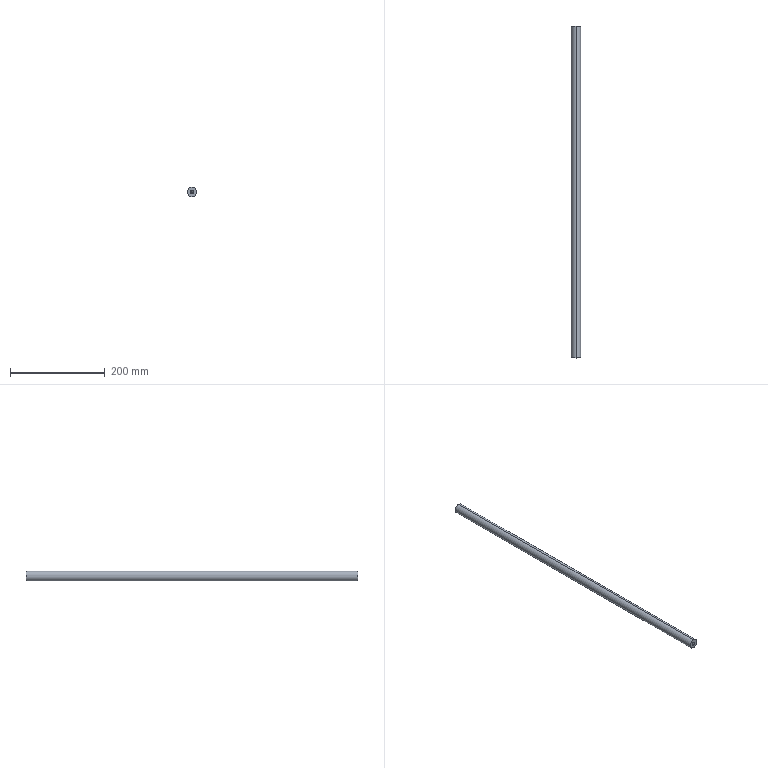Part | SolidWorks | features HoleWzd 2, Extrusion 1 | 1 solid | 12 faces | box 20 x 700 x 20 mm | volume 218428 mm3 | cylinder 6 | cone 4 | plane 2 | commonest cylinder face diameters 6.8 x4 20 x2
STEP:
#1=CARTESIAN_POINT('',(0.,19.75,3.4));
#2=VERTEX_POINT('',#1);
#3=CARTESIAN_POINT('',(0.,19.75,-3.4));
#4=VERTEX_POINT('',#3);
#5=CARTESIAN_POINT('',(0.,19.75,0.));
#6=DIRECTION('',(0.,-1.,0.));
#7=DIRECTION('',(0.,0.,-1.));
#8=AXIS2_PLACEMENT_3D('',#5,#6,#7);
#9=CIRCLE('',#8,3.4);
#10=EDGE_CURVE('',#2,#4,#9,.T.);
#11=ORIENTED_EDGE('',*,*,#10,.F.);
#12=CARTESIAN_POINT('',(0.,0.,3.4));
#13=VERTEX_POINT('',#12);
#14=CARTESIAN_POINT('',(0.,0.,3.4));
#15=DIRECTION('',(0.,-1.,0.));
#16=VECTOR('',#15,1000.);
#17=LINE('',#14,#16);
#18=EDGE_CURVE('',#2,#13,#17,.T.);
#19=ORIENTED_EDGE('',*,*,#18,.T.);
#20=CARTESIAN_POINT('',(0.,0.,-3.4));
#21=VERTEX_POINT('',#20);
#22=CARTESIAN_POINT('',(0.,0.,0.));
#23=DIRECTION('',(0.,-1.,0.));
#24=DIRECTION('',(0.,0.,-1.));
#25=AXIS2_PLACEMENT_3D('',#22,#23,#24);
#26=CIRCLE('',#25,3.4);
#27=EDGE_CURVE('',#13,#21,#26,.T.);
#28=ORIENTED_EDGE('',*,*,#27,.T.);
#29=CARTESIAN_POINT('',(0.,0.,-3.4));
#30=DIRECTION('',(0.,-1.,0.));
#31=VECTOR('',#30,1000.);
#32=LINE('',#29,#31);
#33=EDGE_CURVE('',#4,#21,#32,.T.);
#34=ORIENTED_EDGE('',*,*,#33,.F.);
#35=EDGE_LOOP('',(#11,#19,#28,#34));
#36=FACE_OUTER_BOUND('',#35,.T.);
#37=CARTESIAN_POINT('',(0.,0.,0.));
#38=DIRECTION('',(0.,-1.,0.));
#39=DIRECTION('',(0.,0.,-1.));
#40=AXIS2_PLACEMENT_3D('',#37,#38,#39);
#41=CYLINDRICAL_SURFACE('',#40,3.4);
#42=ADVANCED_FACE('',(#36),#41,.F.);
#43=CARTESIAN_POINT('',(0.,21.793,0.));
#44=VERTEX_POINT('',#43);
#45=CARTESIAN_POINT('',(0.,19.75,-3.4));
#46=DIRECTION('',(0.,-0.515,-0.8572));
#47=VECTOR('',#46,1000.);
#48=LINE('',#45,#47);
#49=EDGE_CURVE('',#44,#4,#48,.T.);
#50=ORIENTED_EDGE('',*,*,#49,.F.);
#51=CARTESIAN_POINT('',(0.,19.75,3.4));
#52=DIRECTION('',(0.,-0.515,0.8572));
#53=VECTOR('',#52,1000.);
#54=LINE('',#51,#53);
#55=EDGE_CURVE('',#44,#2,#54,.T.);
#56=ORIENTED_EDGE('',*,*,#55,.T.);
#57=ORIENTED_EDGE('',*,*,#10,.T.);
#58=EDGE_LOOP('',(#50,#56,#57));
#59=FACE_OUTER_BOUND('',#58,.T.);
#60=CARTESIAN_POINT('',(0.,19.75,0.));
#61=DIRECTION('',(0.,-1.,0.));
#62=DIRECTION('',(0.,0.,-1.));
#63=AXIS2_PLACEMENT_3D('',#60,#61,#62);
#64=CONICAL_SURFACE('',#63,3.4,1.03);
#65=ADVANCED_FACE('',(#59),#64,.F.);
#66=CARTESIAN_POINT('',(0.,680.25,-3.4));
#67=VERTEX_POINT('',#66);
#68=CARTESIAN_POINT('',(0.,680.25,3.4));
#69=VERTEX_POINT('',#68);
#70=CARTESIAN_POINT('',(0.,680.25,0.));
#71=DIRECTION('',(0.,1.,0.));
#72=DIRECTION('',(0.,0.,1.));
#73=AXIS2_PLACEMENT_3D('',#70,#71,#72);
#74=CIRCLE('',#73,3.4);
#75=EDGE_CURVE('',#67,#69,#74,.T.);
#76=ORIENTED_EDGE('',*,*,#75,.F.);
#77=CARTESIAN_POINT('',(0.,700.,-3.4));
#78=VERTEX_POINT('',#77);
#79=CARTESIAN_POINT('',(0.,700.,-3.4));
#80=DIRECTION('',(0.,1.,0.));
#81=VECTOR('',#80,1000.);
#82=LINE('',#79,#81);
#83=EDGE_CURVE('',#67,#78,#82,.T.);
#84=ORIENTED_EDGE('',*,*,#83,.T.);
#85=CARTESIAN_POINT('',(0.,700.,3.4));
#86=VERTEX_POINT('',#85);
#87=CARTESIAN_POINT('',(0.,700.,0.));
#88=DIRECTION('',(0.,1.,0.));
#89=DIRECTION('',(0.,0.,1.));
#90=AXIS2_PLACEMENT_3D('',#87,#88,#89);
#91=CIRCLE('',#90,3.4);
#92=EDGE_CURVE('',#78,#86,#91,.T.);
#93=ORIENTED_EDGE('',*,*,#92,.T.);
#94=CARTESIAN_POINT('',(0.,700.,3.4));
#95=DIRECTION('',(0.,1.,0.));
#96=VECTOR('',#95,1000.);
#97=LINE('',#94,#96);
#98=EDGE_CURVE('',#69,#86,#97,.T.);
#99=ORIENTED_EDGE('',*,*,#98,.F.);
#100=EDGE_LOOP('',(#76,#84,#93,#99));
#101=FACE_OUTER_BOUND('',#100,.T.);
#102=CARTESIAN_POINT('',(0.,700.,0.));
#103=DIRECTION('',(0.,1.,0.));
#104=DIRECTION('',(0.,0.,1.));
#105=AXIS2_PLACEMENT_3D('',#102,#103,#104);
#106=CYLINDRICAL_SURFACE('',#105,3.4);
#107=ADVANCED_FACE('',(#101),#106,.F.);
#108=CARTESIAN_POINT('',(0.,678.207,0.));
#109=VERTEX_POINT('',#108);
#110=CARTESIAN_POINT('',(0.,680.25,3.4));
#111=DIRECTION('',(0.,0.515,0.8572));
#112=VECTOR('',#111,1000.);
#113=LINE('',#110,#112);
#114=EDGE_CURVE('',#109,#69,#113,.T.);
#115=ORIENTED_EDGE('',*,*,#114,.F.);
#116=CARTESIAN_POINT('',(0.,680.25,-3.4));
#117=DIRECTION('',(0.,0.515,-0.8572));
#118=VECTOR('',#117,1000.);
#119=LINE('',#116,#118);
#120=EDGE_CURVE('',#109,#67,#119,.T.);
#121=ORIENTED_EDGE('',*,*,#120,.T.);
#122=ORIENTED_EDGE('',*,*,#75,.T.);
#123=EDGE_LOOP('',(#115,#121,#122));
#124=FACE_OUTER_BOUND('',#123,.T.);
#125=CARTESIAN_POINT('',(0.,680.25,0.));
#126=DIRECTION('',(0.,1.,0.));
#127=DIRECTION('',(0.,0.,1.));
#128=AXIS2_PLACEMENT_3D('',#125,#126,#127);
#129=CONICAL_SURFACE('',#128,3.4,1.03);
#130=ADVANCED_FACE('',(#124),#129,.F.);
#131=CARTESIAN_POINT('',(0.,700.,10.));
#132=VERTEX_POINT('',#131);
#133=CARTESIAN_POINT('',(0.,700.,-10.));
#134=VERTEX_POINT('',#133);
#135=CARTESIAN_POINT('',(0.,700.,0.));
#136=DIRECTION('',(0.,1.,0.));
#137=DIRECTION('',(0.,0.,1.));
#138=AXIS2_PLACEMENT_3D('',#135,#136,#137);
#139=CIRCLE('',#138,10.);
#140=EDGE_CURVE('',#132,#134,#139,.T.);
#141=ORIENTED_EDGE('',*,*,#140,.F.);
#142=CARTESIAN_POINT('',(0.,0.,10.));
#143=VERTEX_POINT('',#142);
#144=CARTESIAN_POINT('',(0.,700.,10.));
#145=DIRECTION('',(0.,-1.,0.));
#146=VECTOR('',#145,1000.);
#147=LINE('',#144,#146);
#148=EDGE_CURVE('',#132,#143,#147,.T.);
#149=ORIENTED_EDGE('',*,*,#148,.T.);
#150=CARTESIAN_POINT('',(0.,0.,-10.));
#151=VERTEX_POINT('',#150);
#152=CARTESIAN_POINT('',(0.,0.,0.));
#153=DIRECTION('',(0.,1.,0.));
#154=DIRECTION('',(0.,0.,1.));
#155=AXIS2_PLACEMENT_3D('',#152,#153,#154);
#156=CIRCLE('',#155,10.);
#157=EDGE_CURVE('',#143,#151,#156,.T.);
#158=ORIENTED_EDGE('',*,*,#157,.T.);
#159=CARTESIAN_POINT('',(0.,700.,-10.));
#160=DIRECTION('',(0.,-1.,0.));
#161=VECTOR('',#160,1000.);
#162=LINE('',#159,#161);
#163=EDGE_CURVE('',#134,#151,#162,.T.);
#164=ORIENTED_EDGE('',*,*,#163,.F.);
#165=EDGE_LOOP('',(#141,#149,#158,#164));
#166=FACE_OUTER_BOUND('',#165,.T.);
#167=CARTESIAN_POINT('',(0.,700.,0.));
#168=DIRECTION('',(0.,-1.,0.));
#169=DIRECTION('',(0.,0.,-1.));
#170=AXIS2_PLACEMENT_3D('',#167,#168,#169);
#171=CYLINDRICAL_SURFACE('',#170,10.);
#172=ADVANCED_FACE('',(#166),#171,.T.);
#173=ORIENTED_EDGE('',*,*,#148,.F.);
#174=CARTESIAN_POINT('',(0.,700.,0.));
#175=DIRECTION('',(0.,1.,0.));
#176=DIRECTION('',(0.,0.,1.));
#177=AXIS2_PLACEMENT_3D('',#174,#175,#176);
#178=CIRCLE('',#177,10.);
#179=EDGE_CURVE('',#134,#132,#178,.T.);
#180=ORIENTED_EDGE('',*,*,#179,.F.);
#181=ORIENTED_EDGE('',*,*,#163,.T.);
#182=CARTESIAN_POINT('',(0.,0.,0.));
#183=DIRECTION('',(0.,1.,0.));
#184=DIRECTION('',(0.,0.,1.));
#185=AXIS2_PLACEMENT_3D('',#182,#183,#184);
#186=CIRCLE('',#185,10.);
#187=EDGE_CURVE('',#151,#143,#186,.T.);
#188=ORIENTED_EDGE('',*,*,#187,.T.);
#189=EDGE_LOOP('',(#173,#180,#181,#188));
#190=FACE_OUTER_BOUND('',#189,.T.);
#191=CARTESIAN_POINT('',(0.,700.,0.));
#192=DIRECTION('',(0.,-1.,0.));
#193=DIRECTION('',(0.,0.,-1.));
#194=AXIS2_PLACEMENT_3D('',#191,#192,#193);
#195=CYLINDRICAL_SURFACE('',#194,10.);
#196=ADVANCED_FACE('',(#190),#195,.T.);
#197=CARTESIAN_POINT('',(0.,700.,0.));
#198=DIRECTION('',(0.,1.,0.));
#199=DIRECTION('',(0.,0.,1.));
#200=AXIS2_PLACEMENT_3D('',#197,#198,#199);
#201=CIRCLE('',#200,3.4);
#202=EDGE_CURVE('',#86,#78,#201,.T.);
#203=ORIENTED_EDGE('',*,*,#202,.F.);
#204=ORIENTED_EDGE('',*,*,#92,.F.);
#205=EDGE_LOOP('',(#203,#204));
#206=FACE_BOUND('',#205,.T.);
#207=ORIENTED_EDGE('',*,*,#179,.T.);
#208=ORIENTED_EDGE('',*,*,#140,.T.);
#209=EDGE_LOOP('',(#207,#208));
#210=FACE_OUTER_BOUND('',#209,.T.);
#211=CARTESIAN_POINT('',(0.,700.,0.));
#212=DIRECTION('',(0.,1.,0.));
#213=DIRECTION('',(0.,0.,1.));
#214=AXIS2_PLACEMENT_3D('',#211,#212,#213);
#215=PLANE('',#214);
#216=ADVANCED_FACE('',(#206,#210),#215,.T.);
#217=CARTESIAN_POINT('',(0.,0.,0.));
#218=DIRECTION('',(0.,-1.,0.));
#219=DIRECTION('',(0.,0.,-1.));
#220=AXIS2_PLACEMENT_3D('',#217,#218,#219);
#221=CIRCLE('',#220,3.4);
#222=EDGE_CURVE('',#21,#13,#221,.T.);
#223=ORIENTED_EDGE('',*,*,#222,.F.);
#224=ORIENTED_EDGE('',*,*,#27,.F.);
#225=EDGE_LOOP('',(#223,#224));
#226=FACE_BOUND('',#225,.T.);
#227=ORIENTED_EDGE('',*,*,#187,.F.);
#228=ORIENTED_EDGE('',*,*,#157,.F.);
#229=EDGE_LOOP('',(#227,#228));
#230=FACE_OUTER_BOUND('',#229,.T.);
#231=CARTESIAN_POINT('',(0.,0.,0.));
#232=DIRECTION('',(0.,1.,0.));
#233=DIRECTION('',(0.,0.,1.));
#234=AXIS2_PLACEMENT_3D('',#231,#232,#233);
#235=PLANE('',#234);
#236=ADVANCED_FACE('',(#226,#230),#235,.F.);
#237=ORIENTED_EDGE('',*,*,#120,.F.);
#238=ORIENTED_EDGE('',*,*,#114,.T.);
#239=CARTESIAN_POINT('',(0.,680.25,0.));
#240=DIRECTION('',(0.,1.,0.));
#241=DIRECTION('',(0.,0.,1.));
#242=AXIS2_PLACEMENT_3D('',#239,#240,#241);
#243=CIRCLE('',#242,3.4);
#244=EDGE_CURVE('',#69,#67,#243,.T.);
#245=ORIENTED_EDGE('',*,*,#244,.T.);
#246=EDGE_LOOP('',(#237,#238,#245));
#247=FACE_OUTER_BOUND('',#246,.T.);
#248=CARTESIAN_POINT('',(0.,680.25,0.));
#249=DIRECTION('',(0.,1.,0.));
#250=DIRECTION('',(0.,0.,1.));
#251=AXIS2_PLACEMENT_3D('',#248,#249,#250);
#252=CONICAL_SURFACE('',#251,3.4,1.03);
#253=ADVANCED_FACE('',(#247),#252,.F.);
#254=ORIENTED_EDGE('',*,*,#83,.F.);
#255=ORIENTED_EDGE('',*,*,#244,.F.);
#256=ORIENTED_EDGE('',*,*,#98,.T.);
#257=ORIENTED_EDGE('',*,*,#202,.T.);
#258=EDGE_LOOP('',(#254,#255,#256,#257));
#259=FACE_OUTER_BOUND('',#258,.T.);
#260=CARTESIAN_POINT('',(0.,700.,0.));
#261=DIRECTION('',(0.,1.,0.));
#262=DIRECTION('',(0.,0.,1.));
#263=AXIS2_PLACEMENT_3D('',#260,#261,#262);
#264=CYLINDRICAL_SURFACE('',#263,3.4);
#265=ADVANCED_FACE('',(#259),#264,.F.);
#266=ORIENTED_EDGE('',*,*,#55,.F.);
#267=ORIENTED_EDGE('',*,*,#49,.T.);
#268=CARTESIAN_POINT('',(0.,19.75,0.));
#269=DIRECTION('',(0.,-1.,0.));
#270=DIRECTION('',(0.,0.,-1.));
#271=AXIS2_PLACEMENT_3D('',#268,#269,#270);
#272=CIRCLE('',#271,3.4);
#273=EDGE_CURVE('',#4,#2,#272,.T.);
#274=ORIENTED_EDGE('',*,*,#273,.T.);
#275=EDGE_LOOP('',(#266,#267,#274));
#276=FACE_OUTER_BOUND('',#275,.T.);
#277=CARTESIAN_POINT('',(0.,19.75,0.));
#278=DIRECTION('',(0.,-1.,0.));
#279=DIRECTION('',(0.,0.,-1.));
#280=AXIS2_PLACEMENT_3D('',#277,#278,#279);
#281=CONICAL_SURFACE('',#280,3.4,1.03);
#282=ADVANCED_FACE('',(#276),#281,.F.);
#283=ORIENTED_EDGE('',*,*,#18,.F.);
#284=ORIENTED_EDGE('',*,*,#273,.F.);
#285=ORIENTED_EDGE('',*,*,#33,.T.);
#286=ORIENTED_EDGE('',*,*,#222,.T.);
#287=EDGE_LOOP('',(#283,#284,#285,#286));
#288=FACE_OUTER_BOUND('',#287,.T.);
#289=CARTESIAN_POINT('',(0.,0.,0.));
#290=DIRECTION('',(0.,-1.,0.));
#291=DIRECTION('',(0.,0.,-1.));
#292=AXIS2_PLACEMENT_3D('',#289,#290,#291);
#293=CYLINDRICAL_SURFACE('',#292,3.4);
#294=ADVANCED_FACE('',(#288),#293,.F.);
#295=CLOSED_SHELL('',(#42,#65,#107,#130,#172,#196,#216,#236,#253,#265,#282,#294));
#296=MANIFOLD_SOLID_BREP('',#295);
#297=CARTESIAN_POINT('',(0.,0.,0.));
#298=DIRECTION('',(0.,0.,1.));
#299=DIRECTION('',(1.,0.,0.));
#300=AXIS2_PLACEMENT_3D('',#297,#298,#299);
#301=(LENGTH_UNIT()NAMED_UNIT(*)SI_UNIT(.MILLI.,.METRE.));
#302=UNCERTAINTY_MEASURE_WITH_UNIT(LENGTH_MEASURE(0.00001),#301,'','');
#303=(NAMED_UNIT(*)PLANE_ANGLE_UNIT()SI_UNIT($,.RADIAN.));
#304=(NAMED_UNIT(*)SI_UNIT($,.STERADIAN.)SOLID_ANGLE_UNIT());
#305=(GEOMETRIC_REPRESENTATION_CONTEXT(3)GLOBAL_UNCERTAINTY_ASSIGNED_CONTEXT((#302))GLOBAL_UNIT_ASSIGNED_CONTEXT((#301,#303,#304))REPRESENTATION_CONTEXT('',''));
#306=ADVANCED_BREP_SHAPE_REPRESENTATION('',(#296,#300),#305);